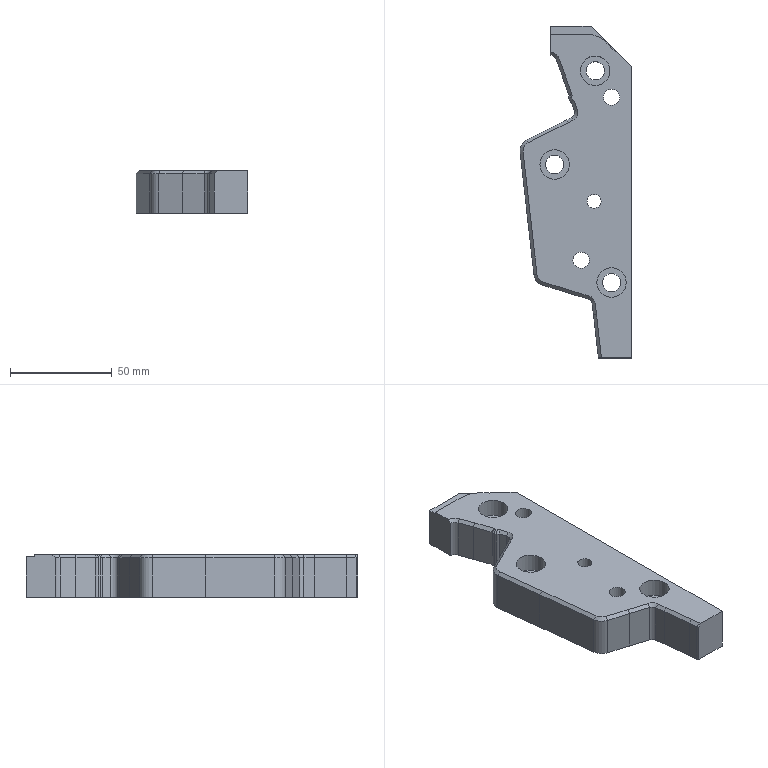Part | NX | features 23 2 | 1 solid | 68 faces | box 54.926 x 163 x 21 mm | volume 120870 mm3 | plane 40 | cylinder 19 | cone 9 | commonest cylinder face diameters 9 x3 14.5 x3 4.4 x2 5.6 x2 8.001 x2 12.4 x2